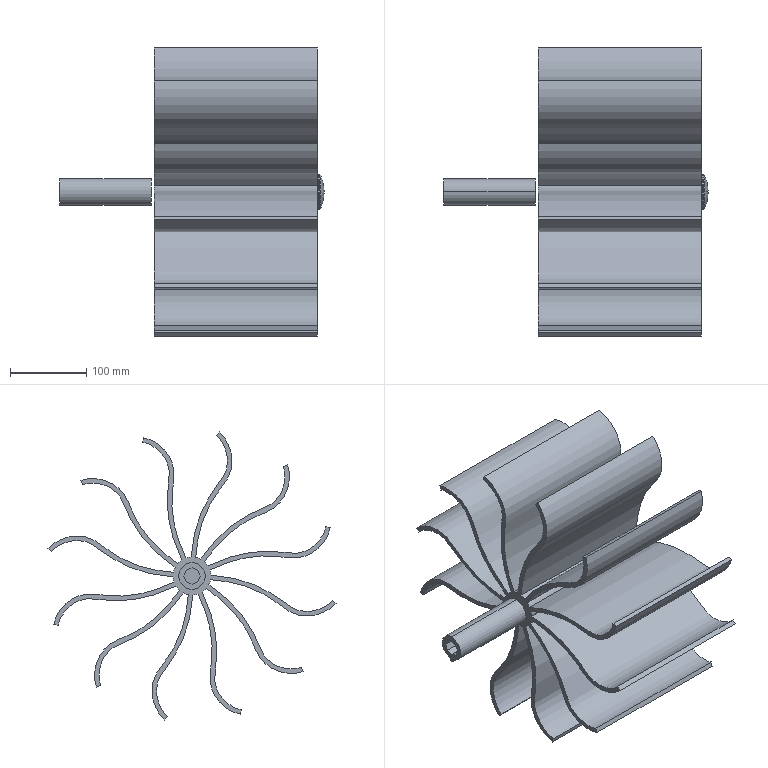Part | STEP file | lopatki1V11 | 2 solids | 83 faces | box 347 x 377.952 x 377.952 mm | volume 3263464 mm3 | plane 37 | spline 24 | cylinder 16 | torus 4 | sphere 2 | commonest cylinder face diameters 50 x12 35 x2 45 x2